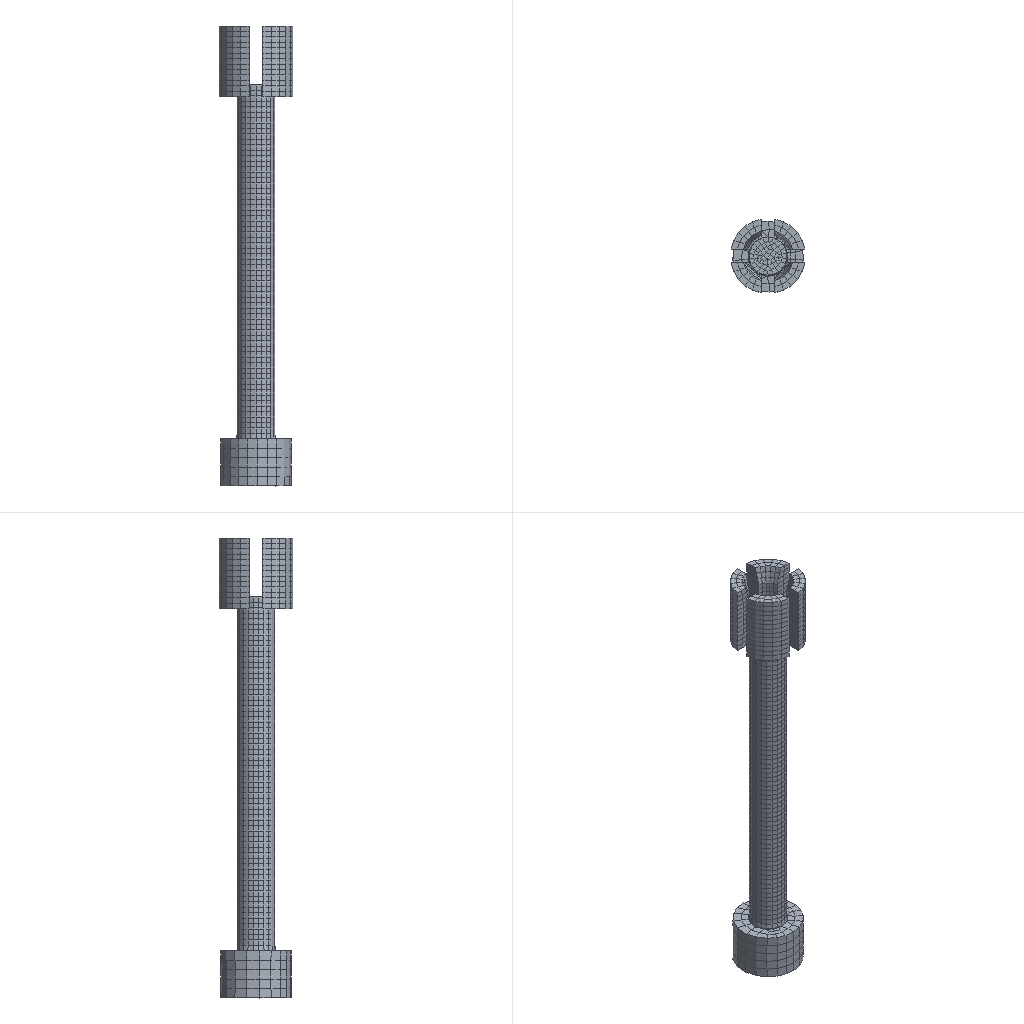Simulation study | abaqus
Set-up summary:
category,name,step,type,value,unit,region
solver,abaqus
solver,version,,,Abaqus/Explicit 2020
units,not stated in the deck,,not stated
analysis,deck,,dynamic temperature-displacement,dynamic temperature-displacement
load_step,Step-1,Step-1,dynamic temperature-displacement,nlgeom=True
contact,interactions,,,general=1 pairs=0 ties=1
load_step,requested,,,1
mesh,nodes,,,6411
mesh,elements,,,5446
element_type,S3,,shell,4
element_type,S4R,,shell,268
element_type,S4RT,,shell,808
element_type,C3D8RT,,solid,4366
load,load commands in deck,,count,6
bc,support commands in deck,,count,12
material,W,,in results
check,setup vs results,,match,"per instance, exact: element labels, types and connectivity; labels of the nodes the elements use; coordinates of those nodes at SINGLE_PRECISION in 5 of 6 instance(s)"
Abaqus input file, long lists of numbers shortened:
*Heading
** Job name: Job-1 Model name: Model-1
** Generated by: Abaqus/CAE 2020
*Preprint, echo=NO, model=NO, history=NO, contact=NO
**
** PARTS
**
*Part, name=work-1
*Node
      1,           0.,           8.,          20.
      2,           0.,           8.,         170.
** (5323 more lines like these left out)
*Element, type=C3D8RT
   1,    1,  100,  101,   24,  165, 1831, 1832,  186
   2,  105,   84,   22,   23, 1836, 1815,  184,  185
** (4364 more lines like these left out)
*Nset, nset=Set-2, generate
    1,  5325,     1
*Elset, elset=Set-2, generate
    1,  4366,     1
** Section: w
*Solid Section, elset=Set-2, material=w
,
*End Part
**
*Part, name=work-2
*Node
      1,           0.,          15.,           0.
      2,           0.,          15.,          20.
** (268 more lines like these left out)
*Element, type=S4R
  1,  15,  71,  79,  14
  2,  71,  72,  80,  79
** (266 more lines like these left out)
*Element, type=S3
220,   3, 214, 226
221,  52, 228, 227
** (2 more lines like these left out)
*Nset, nset=Set-2, generate
   1,  270,    1
*Elset, elset=Set-2, generate
   1,  272,    1
** Section: Section-3
*Shell Section, elset=Set-2, material=w
1., 5
*End Part
**
*Part, name=work-3
*Node
      1,   15.545,  -2.907,         215.
      2,   15.545,  -2.907,         185.
** (202 more lines like these left out)
*Element, type=S4RT
 1,  1, 13, 85, 36
 2, 13, 14, 86, 85
** (200 more lines like these left out)
*Nset, nset=Set-2, generate
   1,  204,    1
*Elset, elset=Set-2, generate
   1,  202,    1
** Section: Section-3
*Shell Section, elset=Set-2, material=w
1., 5
*End Part
**
*Part, name=work-4
*Node
      1,  -2.907,  -15.545,         215.
      2,  -2.907,  -15.545,         185.
** (202 more lines like these left out)
*Element, type=S4RT
 1,  1, 13, 85, 36
 2, 13, 14, 86, 85
** (200 more lines like these left out)
*Nset, nset=Set-2, generate
   1,  204,    1
*Elset, elset=Set-2, generate
   1,  202,    1
** Section: Section-3
*Shell Section, elset=Set-2, material=w
1., 5
*End Part
**
*Part, name=work-5
*Node
      1,  -15.545,   2.907,         215.
      2,  -15.545,   2.907,         185.
** (202 more lines like these left out)
*Element, type=S4RT
 1,  1, 13, 85, 36
 2, 13, 14, 86, 85
** (200 more lines like these left out)
*Nset, nset=Set-2, generate
   1,  204,    1
*Elset, elset=Set-2, generate
   1,  202,    1
** Section: Section-3
*Shell Section, elset=Set-2, material=w
1., 5
*End Part
**
*Part, name=work-6
*Node
      1,   2.907,   15.545,         215.
      2,   2.907,   15.545,         185.
** (202 more lines like these left out)
*Element, type=S4RT
 1,  1, 13, 85, 36
 2, 13, 14, 86, 85
** (200 more lines like these left out)
*Nset, nset=Set-3, generate
   1,  204,    1
*Elset, elset=Set-3, generate
   1,  202,    1
** Section: Section-3
*Shell Section, elset=Set-3, material=w
1., 5
*End Part
**
**
** ASSEMBLY
**
*Assembly, name=Assembly
**
*Instance, name=work-1-1, part=work-1
*End Instance
**
*Instance, name=work-2-1, part=work-2
*End Instance
**
*Instance, name=work-3-1, part=work-3
          0.,           0.,         -20.
*End Instance
**
*Instance, name=work-4-1, part=work-4
          0.,           0.,         -20.
*End Instance
**
*Instance, name=work-5-1, part=work-5
          0.,           0.,         -20.
*End Instance
**
*Instance, name=work-6-1, part=work-6
          0.,           0.,         -20.
*End Instance
**
*Node
      1,           0., 9.18485047e-16,           0.
*Node
      2,           0., 4.4408921e-16,        187.5
*Node
      3,  -6.364,   6.364,        187.5
*Node
      4,   6.364,   6.364,        187.5
*Node
      5,   6.364,  -6.364,        187.5
*Node
      6,  -6.364,  -6.364,        187.5
*Element, type=CONN3D2
1, 2, 3
*Connector Section, elset=Set-17
Slide-Plane, Revolute
"Datum csys-2_Set-17-1_",
*Element, type=CONN3D2
2, 2, 4
*Connector Section, elset=Set-19
Slide-Plane, Revolute
"Datum csys-2_Set-19-1_",
*Element, type=CONN3D2
3, 2, 5
*Connector Section, elset=Set-21
Slide-Plane, Revolute
"Datum csys-2_Set-21-1_",
*Element, type=CONN3D2
4, 2, 6
*Connector Section, elset=Set-23
Slide-Plane, Revolute
"Datum csys-2_Set-23-1_",
*Nset, nset=Set-1, instance=work-1-1, generate
    1,  5325,     1
*Nset, nset=Set-1, instance=work-2-1, generate
   1,  270,    1
*Nset, nset=Set-1, instance=work-4-1, generate
   1,  204,    1
*Nset, nset=Set-1, instance=work-6-1, generate
   1,  204,    1
*Nset, nset=Set-1, instance=work-3-1, generate
   1,  204,    1
*Nset, nset=Set-1, instance=work-5-1, generate
   1,  204,    1
*Elset, elset=Set-1, instance=work-1-1, generate
    1,  4366,     1
*Elset, elset=Set-1, instance=work-2-1, generate
   1,  272,    1
*Elset, elset=Set-1, instance=work-4-1, generate
   1,  202,    1
*Elset, elset=Set-1, instance=work-6-1, generate
   1,  202,    1
*Elset, elset=Set-1, instance=work-3-1, generate
   1,  202,    1
*Elset, elset=Set-1, instance=work-5-1, generate
   1,  202,    1
*Nset, nset=Set-4
 1,
*Nset, nset=Set-17
 2, 3
*Elset, elset=Set-17
 1,
*Nset, nset=Set-19
 2, 4
*Elset, elset=Set-19
 2,
*Nset, nset=Set-21
 2, 5
*Elset, elset=Set-21
 3,
*Nset, nset=Set-23
 2, 6
*Elset, elset=Set-23
 4,
*Nset, nset=Set-24, generate
 2,  6,  1
*Elset, elset=Set-24, generate
 1,  4,  1
*Nset, nset=Set-25
 2, 3
*Elset, elset=Set-25
 1,
*Nset, nset=Set-26
 2, 4
*Elset, elset=Set-26
 2,
*Nset, nset=Set-27
 2, 5
*Elset, elset=Set-27
 3,
*Nset, nset=Set-28
 2, 6
*Elset, elset=Set-28
 4,
*Nset, nset=Set-29, instance=work-2-1, generate
   1,  270,    1
*Nset, nset=Set-29, instance=work-3-1, generate
   1,  204,    1
*Nset, nset=Set-29, instance=work-4-1, generate
   1,  204,    1
*Nset, nset=Set-29, instance=work-6-1, generate
   1,  204,    1
*Nset, nset=Set-29, instance=work-5-1, generate
   1,  204,    1
*Elset, elset=Set-29, instance=work-2-1, generate
   1,  272,    1
*Elset, elset=Set-29, instance=work-3-1, generate
   1,  202,    1
*Elset, elset=Set-29, instance=work-4-1, generate
   1,  202,    1
*Elset, elset=Set-29, instance=work-6-1, generate
   1,  202,    1
*Elset, elset=Set-29, instance=work-5-1, generate
   1,  202,    1
*Nset, nset=Set-30, instance=work-1-1, generate
    1,  5325,     1
*Elset, elset=Set-30, instance=work-1-1, generate
    1,  4366,     1
*Nset, nset=Set-31
 2,
*Nset, nset=Wire-1-Set-2
 2, 3
*Elset, elset=Wire-1-Set-2
 1,
*Nset, nset=Wire-2-Set-1
 2, 4
*Elset, elset=Wire-2-Set-1
 2,
*Nset, nset=Wire-3-Set-1
 2, 5
*Elset, elset=Wire-3-Set-1
 3,
*Nset, nset=Wire-4-Set-1
 2, 6
*Elset, elset=Wire-4-Set-1
 4,
*Nset, nset=b_Set-2, instance=work-2-1, generate
   1,  270,    1
*Elset, elset=b_Set-2, instance=work-2-1, generate
   1,  272,    1
*Nset, nset=b_Set-5, instance=work-5-1, generate
   1,  204,    1
*Elset, elset=b_Set-5, instance=work-5-1, generate
   1,  202,    1
*Nset, nset=b_Set-7, instance=work-6-1, generate
   1,  204,    1
*Elset, elset=b_Set-7, instance=work-6-1, generate
   1,  202,    1
*Nset, nset=b_Set-9, instance=work-3-1, generate
   1,  204,    1
*Elset, elset=b_Set-9, instance=work-3-1, generate
   1,  202,    1
*Nset, nset=b_Set-11, instance=work-4-1, generate
   1,  204,    1
*Elset, elset=b_Set-11, instance=work-4-1, generate
   1,  202,    1
*Nset, nset=_PickedSet19, internal
 1,
*Nset, nset=_PickedSet28, internal
 3,
*Nset, nset=_PickedSet30, internal
 4,
*Nset, nset=_PickedSet32, internal
 5,
*Nset, nset=_PickedSet34, internal
 6,
*Elset, elset=_m_Surf-1_SPOS, internal, instance=work-2-1, generate
 106,  175,    1
*Surface, type=ELEMENT, name=m_Surf-1
_m_Surf-1_SPOS, SPOS
*Elset, elset=_m_Surf-3_SPOS, internal, instance=work-5-1, generate
 27,  61,   1
*Surface, type=ELEMENT, name=m_Surf-3
_m_Surf-3_SPOS, SPOS
*Elset, elset=_m_Surf-5_SPOS, internal, instance=work-6-1, generate
 27,  61,   1
*Surface, type=ELEMENT, name=m_Surf-5
_m_Surf-5_SPOS, SPOS
*Elset, elset=_m_Surf-6_SPOS, internal, instance=work-3-1, generate
 27,  61,   1
*Surface, type=ELEMENT, name=m_Surf-6
_m_Surf-6_SPOS, SPOS
*Elset, elset=_m_Surf-7_SPOS, internal, instance=work-4-1, generate
 27,  61,   1
*Surface, type=ELEMENT, name=m_Surf-7
_m_Surf-7_SPOS, SPOS
*Elset, elset=_s_Surf-1_S3, internal, instance=work-1-1
 3836, 3841, 3855, 3889, 3895, 3900, 3914, 3948, 3954, 3959, 3973, 4007, 4013, 4018, 4032, 4066
 4072, 4077, 4091, 4125, 4131, 4136, 4150, 4184, 4190, 4195, 4209, 4243, 4249, 4254, 4268, 4302
** (1 more lines like these left out)
*Elset, elset=_s_Surf-1_S4, internal, instance=work-1-1
 3837, 3846, 3861, 3869, 3896, 3905, 3920, 3928, 3955, 3964, 3979, 3987, 4014, 4023, 4038, 4046
 4073, 4082, 4097, 4105, 4132, 4141, 4156, 4164, 4191, 4200, 4215, 4223, 4250, 4259, 4274, 4282
** (1 more lines like these left out)
*Elset, elset=_s_Surf-1_S5, internal, instance=work-1-1
 3845, 3847, 3850, 3856, 3857, 3858, 3859, 3860, 3863, 3865, 3870, 3904, 3906, 3909, 3915, 3916
 3917, 3918, 3919, 3922, 3924, 3929, 3963, 3965, 3968, 3974, 3975, 3976, 3977, 3978, 3981, 3983
** (5 more lines like these left out)
*Elset, elset=_s_Surf-1_S6, internal, instance=work-1-1
 3862, 3868, 3873, 3921, 3927, 3932, 3980, 3986, 3991, 4039, 4045, 4050, 4098, 4104, 4109, 4157
 4163, 4168, 4216, 4222, 4227, 4275, 4281, 4286, 4334, 4340, 4345
*Surface, type=ELEMENT, name=s_Surf-1
_s_Surf-1_S3, S3
_s_Surf-1_S4, S4
_s_Surf-1_S6, S6
_s_Surf-1_S5, S5
*Elset, elset=_s_Surf-3_S6, internal, instance=work-1-1
    1,    6,   20,   54,   60,   65,   79,  113,  119,  124,  138,  172,  178,  183,  197,  231
  237,  242,  256,  290,  296,  301,  315,  349,  355,  360,  374,  408,  414,  419,  433,  467
** (15 more lines like these left out)
*Elset, elset=_s_Surf-3_S5, internal, instance=work-1-1
    2,   11,   26,   34,   61,   70,   85,   93,  120,  129,  144,  152,  179,  188,  203,  211
  238,  247,  262,  270,  297,  306,  321,  329,  356,  365,  380,  388,  415,  424,  439,  447
** (15 more lines like these left out)
*Elset, elset=_s_Surf-3_S4, internal, instance=work-1-1
   10,   12,   15,   21,   22,   23,   24,   25,   28,   30,   35,   69,   71,   74,   80,   81
   82,   83,   84,   87,   89,   94,  128,  130,  133,  139,  140,  141,  142,  143,  146,  148
** (43 more lines like these left out)
*Elset, elset=_s_Surf-3_S3, internal, instance=work-1-1
   27,   33,   38,   86,   92,   97,  145,  151,  156,  204,  210,  215,  263,  269,  274,  322
  328,  333,  381,  387,  392,  440,  446,  451,  499,  505,  510,  558,  564,  569,  617,  623
** (11 more lines like these left out)
*Surface, type=ELEMENT, name=s_Surf-3
_s_Surf-3_S6, S6
_s_Surf-3_S5, S5
_s_Surf-3_S4, S4
_s_Surf-3_S3, S3
*Orientation, name="Datum csys-2_Set-17-1_"
          0.,           0.,          -1.,           0.,          -1.,           0.
1, 45.
*Orientation, name="Datum csys-2_Set-19-1_"
          0.,           0.,          -1.,           0.,          -1.,           0.
1, 135.
*Orientation, name="Datum csys-2_Set-21-1_"
          0.,           0.,          -1.,           0.,          -1.,           0.
1, 225.
*Orientation, name="Datum csys-2_Set-23-1_"
          0.,           0.,          -1.,           0.,          -1.,           0.
1, -45.
** Constraint: Constraint-1
*Tie, name=Constraint-1, adjust=yes
s_Surf-1, m_Surf-1
** Constraint: Constraint-2
*Rigid Body, ref node=_PickedSet19, elset=b_Set-2
** Constraint: Constraint-3
*Rigid Body, ref node=_PickedSet28, elset=b_Set-5
** Constraint: Constraint-4
*Rigid Body, ref node=_PickedSet30, elset=b_Set-7
** Constraint: Constraint-5
*Rigid Body, ref node=_PickedSet32, elset=b_Set-9
** Constraint: Constraint-6
*Rigid Body, ref node=_PickedSet34, elset=b_Set-11
*End Assembly
*Amplitude, name=Amp-1
             0.,              0.,             0.3,              1.
*Amplitude, name=Amp-2, definition=PERIODIC
1,            62.8,              0.,              0.
        124.658,              0.
**
** MATERIALS
**
*Material, name=w
*Conductivity
162.,
*Density
 1.7e-08,
*Elastic
320000., 0.28
*Expansion
 0.005,
*Plastic
1500.,0.
*Specific Heat
 1.34e+08,
**
** INTERACTION PROPERTIES
**
*Surface Interaction, name=IntProp-1
*Friction
 0.01,
*Surface Behavior, pressure-overclosure=HARD
**
** PREDEFINED FIELDS
**
** Name: Predefined Field-1   Type: Temperature
*Initial Conditions, type=TEMPERATURE
Set-29, 20., 20., 20., 20., 20.
** Name: Predefined Field-2   Type: Temperature
*Initial Conditions, type=TEMPERATURE
Set-30, 900., 900., 900., 900., 900.
** ----------------------------------------------------------------
**
** STEP: Step-1
**
*Step, name=Step-1, nlgeom=YES
*Dynamic Temperature-displacement, Explicit
, 0.2
*Bulk Viscosity
0.06, 1.2
** Mass Scaling: Semi-Automatic
**               Whole Model
*Fixed Mass Scaling, factor=50.
**
** BOUNDARY CONDITIONS
**
** Name: BC-2 Type: 连接速度
*Connector Motion, type=VELOCITY
Set-24, 4
** Name: BC-3 Type: 连接速度
*Connector Motion, amplitude=Amp-2, type=VELOCITY
Set-25, 2
Set-25, 3, 1.
** Name: BC-4 Type: 连接速度
*Connector Motion, amplitude=Amp-2, type=VELOCITY
Set-26, 2
Set-26, 3, 1.
** Name: BC-5 Type: 连接速度
*Connector Motion, amplitude=Amp-2, type=VELOCITY
Set-27, 2
Set-27, 3, 1.
** Name: BC-6 Type: 连接速度
*Connector Motion, amplitude=Amp-2, type=VELOCITY
Set-28, 2
Set-28, 3, 1.
** Name: BC-7 Type: 速度/角速度
*Boundary, type=VELOCITY
Set-31, 1, 1
Set-31, 2, 2
Set-31, 3, 3
Set-31, 4, 4
Set-31, 5, 5
Set-31, 6, 6, 6.28
** Name: [REDACTED] : Displacement/rotation angle
*Boundary, amplitude=Amp-1
Set-4, 1, 1
Set-4, 2, 2
Set-4, 3, 3, 50.
Set-4, 4, 4
Set-4, 5, 5
Set-4, 6, 6
**
** INTERACTIONS
**
** Interaction: Int-5
*Contact, op=NEW
*Contact Inclusions, ALL EXTERIOR
*Contact Property Assignment
 ,  , IntProp-1
**
** OUTPUT REQUESTS
**
*Restart, write, number interval=1, time marks=NO
**
** FIELD OUTPUT: F-Output-1
**
*Output, field, number interval=50
*Node Output
A, CF, NT, RF, RFL, RM, RT, U
V
*Element Output, directions=YES
E, EVF, HFL, LE, MISES, MISESMAX, MISESONLY, NE, P, PE, PEEQ, PEEQMAX, PEEQT, PEEQVAVG, PEMAG, PEVAVG
PRESSONLY, S, SEQUT, SF, SSAVG, SVAVG, TEMP, YIELDPOT
*Contact Output
CDISP, CFORCE, CSTRESS, FSLIP, FSLIPR, PPRESS
**
** HISTORY OUTPUT: H-Output-1
**
*Output, history, variable=PRESELECT
*End Step
Results summary:
result,step,Step-1,completed,increments=119565 time=0.2/0.2
result,analysis,,,"dynamic temperature-displacement, explict"
result,last_loadstep,,,1
result,analysis steps,,count,1
result,primary field,,,"U, UR, NT11"
result,reaction total,,FX,-16069.82,model units
result,reaction total,,FY,-179382.224,model units
result,reaction total,,FZ,-2708.104,model units